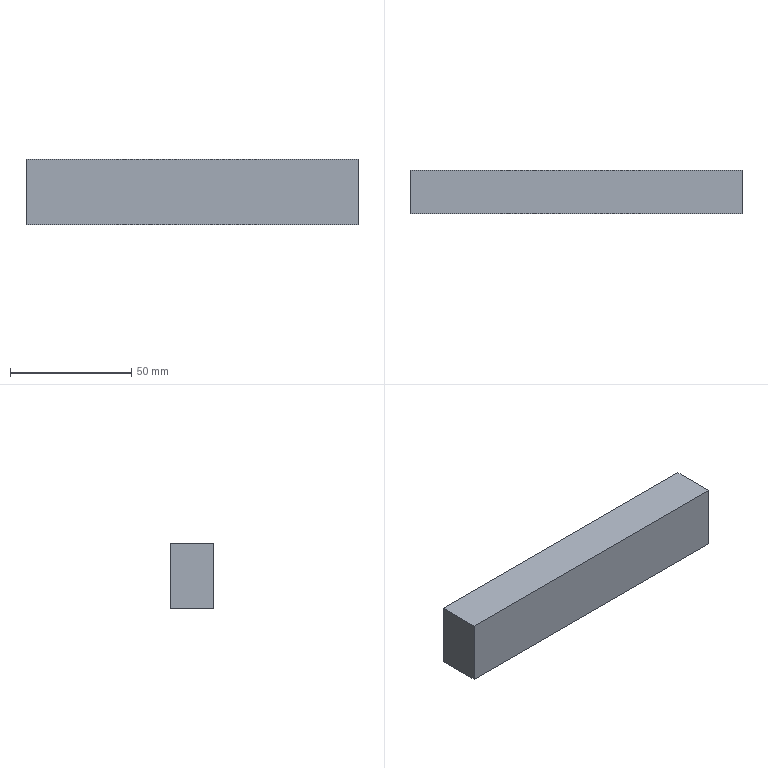Part | NX | 1 solid | 6 faces | box 137.023 x 18 x 26.957 mm | volume 66486 mm3 | plane 6
STEP:
#1=CARTESIAN_POINT('',(-187.326,-727.347,2346.265));
#2=VERTEX_POINT('',#1);
#3=CARTESIAN_POINT('',(-187.326,-727.347,2373.222));
#4=VERTEX_POINT('',#3);
#5=CARTESIAN_POINT('',(-187.326,-727.347,2346.265));
#6=DIRECTION('',(0.,0.,1.));
#7=VECTOR('',#6,1.);
#8=LINE('',#5,#7);
#9=EDGE_CURVE('',#2,#4,#8,.T.);
#10=ORIENTED_EDGE('',*,*,#9,.T.);
#11=CARTESIAN_POINT('',(-187.326,-709.347,2373.222));
#12=VERTEX_POINT('',#11);
#13=CARTESIAN_POINT('',(-187.326,-709.347,2373.222));
#14=DIRECTION('',(0.,-1.,0.));
#15=VECTOR('',#14,1.);
#16=LINE('',#13,#15);
#17=EDGE_CURVE('',#12,#4,#16,.T.);
#18=ORIENTED_EDGE('',*,*,#17,.F.);
#19=CARTESIAN_POINT('',(-187.326,-709.347,2346.265));
#20=VERTEX_POINT('',#19);
#21=CARTESIAN_POINT('',(-187.326,-709.347,2346.265));
#22=DIRECTION('',(0.,0.,1.));
#23=VECTOR('',#22,1.);
#24=LINE('',#21,#23);
#25=EDGE_CURVE('',#20,#12,#24,.T.);
#26=ORIENTED_EDGE('',*,*,#25,.F.);
#27=CARTESIAN_POINT('',(-187.326,-709.347,2346.265));
#28=DIRECTION('',(0.,-1.,0.));
#29=VECTOR('',#28,1.);
#30=LINE('',#27,#29);
#31=EDGE_CURVE('',#20,#2,#30,.T.);
#32=ORIENTED_EDGE('',*,*,#31,.T.);
#33=EDGE_LOOP('',(#10,#18,#26,#32));
#34=FACE_OUTER_BOUND('',#33,.T.);
#35=CARTESIAN_POINT('',(-187.326,-709.347,2346.265));
#36=DIRECTION('',(1.,0.,0.));
#37=DIRECTION('',(0.,0.,-1.));
#38=AXIS2_PLACEMENT_3D('',#35,#36,#37);
#39=PLANE('',#38);
#40=ADVANCED_FACE('',(#34),#39,.F.);
#41=CARTESIAN_POINT('',(-50.304,-727.347,2373.222));
#42=VERTEX_POINT('',#41);
#43=CARTESIAN_POINT('',(-187.326,-727.347,2373.222));
#44=DIRECTION('',(1.,0.,0.));
#45=VECTOR('',#44,1.);
#46=LINE('',#43,#45);
#47=EDGE_CURVE('',#4,#42,#46,.T.);
#48=ORIENTED_EDGE('',*,*,#47,.T.);
#49=CARTESIAN_POINT('',(-50.304,-709.347,2373.222));
#50=VERTEX_POINT('',#49);
#51=CARTESIAN_POINT('',(-50.304,-709.347,2373.222));
#52=DIRECTION('',(0.,-1.,0.));
#53=VECTOR('',#52,1.);
#54=LINE('',#51,#53);
#55=EDGE_CURVE('',#50,#42,#54,.T.);
#56=ORIENTED_EDGE('',*,*,#55,.F.);
#57=CARTESIAN_POINT('',(-187.326,-709.347,2373.222));
#58=DIRECTION('',(1.,0.,0.));
#59=VECTOR('',#58,1.);
#60=LINE('',#57,#59);
#61=EDGE_CURVE('',#12,#50,#60,.T.);
#62=ORIENTED_EDGE('',*,*,#61,.F.);
#63=ORIENTED_EDGE('',*,*,#17,.T.);
#64=EDGE_LOOP('',(#48,#56,#62,#63));
#65=FACE_OUTER_BOUND('',#64,.T.);
#66=CARTESIAN_POINT('',(-187.326,-709.347,2373.222));
#67=DIRECTION('',(0.,0.,-1.));
#68=DIRECTION('',(-1.,0.,0.));
#69=AXIS2_PLACEMENT_3D('',#66,#67,#68);
#70=PLANE('',#69);
#71=ADVANCED_FACE('',(#65),#70,.F.);
#72=CARTESIAN_POINT('',(-50.304,-727.347,2346.265));
#73=VERTEX_POINT('',#72);
#74=CARTESIAN_POINT('',(-50.304,-727.347,2346.265));
#75=DIRECTION('',(0.,0.,-1.));
#76=VECTOR('',#75,1.);
#77=LINE('',#74,#76);
#78=EDGE_CURVE('',#42,#73,#77,.T.);
#79=ORIENTED_EDGE('',*,*,#78,.T.);
#80=CARTESIAN_POINT('',(-50.304,-709.347,2346.265));
#81=VERTEX_POINT('',#80);
#82=CARTESIAN_POINT('',(-50.304,-709.347,2346.265));
#83=DIRECTION('',(0.,-1.,0.));
#84=VECTOR('',#83,1.);
#85=LINE('',#82,#84);
#86=EDGE_CURVE('',#81,#73,#85,.T.);
#87=ORIENTED_EDGE('',*,*,#86,.F.);
#88=CARTESIAN_POINT('',(-50.304,-709.347,2346.265));
#89=DIRECTION('',(0.,0.,-1.));
#90=VECTOR('',#89,1.);
#91=LINE('',#88,#90);
#92=EDGE_CURVE('',#50,#81,#91,.T.);
#93=ORIENTED_EDGE('',*,*,#92,.F.);
#94=ORIENTED_EDGE('',*,*,#55,.T.);
#95=EDGE_LOOP('',(#79,#87,#93,#94));
#96=FACE_OUTER_BOUND('',#95,.T.);
#97=CARTESIAN_POINT('',(-50.304,-709.347,2346.265));
#98=DIRECTION('',(-1.,0.,0.));
#99=DIRECTION('',(0.,0.,1.));
#100=AXIS2_PLACEMENT_3D('',#97,#98,#99);
#101=PLANE('',#100);
#102=ADVANCED_FACE('',(#96),#101,.F.);
#103=CARTESIAN_POINT('',(-187.326,-727.347,2346.265));
#104=DIRECTION('',(-1.,0.,0.));
#105=VECTOR('',#104,1.);
#106=LINE('',#103,#105);
#107=EDGE_CURVE('',#73,#2,#106,.T.);
#108=ORIENTED_EDGE('',*,*,#107,.T.);
#109=ORIENTED_EDGE('',*,*,#31,.F.);
#110=CARTESIAN_POINT('',(-187.326,-709.347,2346.265));
#111=DIRECTION('',(-1.,0.,0.));
#112=VECTOR('',#111,1.);
#113=LINE('',#110,#112);
#114=EDGE_CURVE('',#81,#20,#113,.T.);
#115=ORIENTED_EDGE('',*,*,#114,.F.);
#116=ORIENTED_EDGE('',*,*,#86,.T.);
#117=EDGE_LOOP('',(#108,#109,#115,#116));
#118=FACE_OUTER_BOUND('',#117,.T.);
#119=CARTESIAN_POINT('',(-187.326,-709.347,2346.265));
#120=DIRECTION('',(0.,0.,1.));
#121=DIRECTION('',(1.,0.,0.));
#122=AXIS2_PLACEMENT_3D('',#119,#120,#121);
#123=PLANE('',#122);
#124=ADVANCED_FACE('',(#118),#123,.F.);
#125=ORIENTED_EDGE('',*,*,#25,.T.);
#126=ORIENTED_EDGE('',*,*,#61,.T.);
#127=ORIENTED_EDGE('',*,*,#92,.T.);
#128=ORIENTED_EDGE('',*,*,#114,.T.);
#129=EDGE_LOOP('',(#125,#126,#127,#128));
#130=FACE_OUTER_BOUND('',#129,.T.);
#131=CARTESIAN_POINT('',(-187.326,-709.347,2373.222));
#132=DIRECTION('',(0.,1.,0.));
#133=DIRECTION('',(0.,0.,1.));
#134=AXIS2_PLACEMENT_3D('',#131,#132,#133);
#135=PLANE('',#134);
#136=ADVANCED_FACE('',(#130),#135,.T.);
#137=ORIENTED_EDGE('',*,*,#9,.F.);
#138=ORIENTED_EDGE('',*,*,#107,.F.);
#139=ORIENTED_EDGE('',*,*,#78,.F.);
#140=ORIENTED_EDGE('',*,*,#47,.F.);
#141=EDGE_LOOP('',(#137,#138,#139,#140));
#142=FACE_OUTER_BOUND('',#141,.T.);
#143=CARTESIAN_POINT('',(-187.326,-727.347,2373.222));
#144=DIRECTION('',(0.,1.,0.));
#145=DIRECTION('',(0.,0.,1.));
#146=AXIS2_PLACEMENT_3D('',#143,#144,#145);
#147=PLANE('',#146);
#148=ADVANCED_FACE('',(#142),#147,.F.);
#149=CLOSED_SHELL('',(#40,#71,#102,#124,#136,#148));
#150=MANIFOLD_SOLID_BREP('',#149);
#151=(LENGTH_UNIT()NAMED_UNIT(*)SI_UNIT(.MILLI.,.METRE.));
#152=UNCERTAINTY_MEASURE_WITH_UNIT(LENGTH_MEASURE(0.00002),#151,'','');
#153=(NAMED_UNIT(*)PLANE_ANGLE_UNIT()SI_UNIT($,.RADIAN.));
#154=PLANE_ANGLE_MEASURE_WITH_UNIT(PLANE_ANGLE_MEASURE(0.01745),#153);
#155=DIMENSIONAL_EXPONENTS(0.,0.,0.,0.,0.,0.,0.);
#156=(CONVERSION_BASED_UNIT('DEGREE',#154)NAMED_UNIT(#155)PLANE_ANGLE_UNIT());
#157=(NAMED_UNIT(*)SI_UNIT($,.STERADIAN.)SOLID_ANGLE_UNIT());
#158=(GEOMETRIC_REPRESENTATION_CONTEXT(3)GLOBAL_UNCERTAINTY_ASSIGNED_CONTEXT((#152))GLOBAL_UNIT_ASSIGNED_CONTEXT((#151,#156,#157))REPRESENTATION_CONTEXT('',''));
#159=ADVANCED_BREP_SHAPE_REPRESENTATION('',(#150),#158);